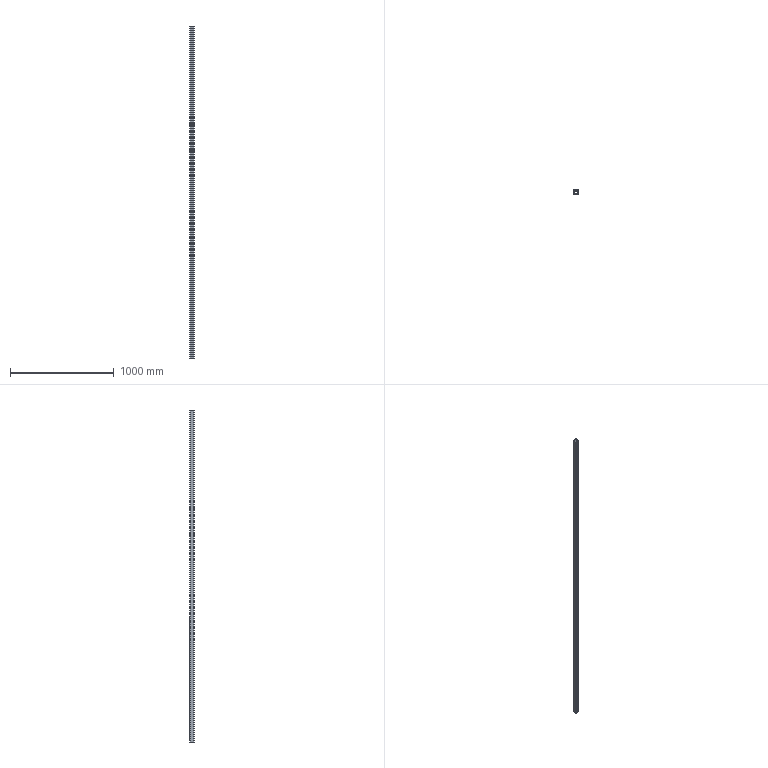Part | NX | features BREP 1 | 1 solid | 102 faces | box 40 x 42 x 3200 mm | volume 1980279 mm3 | plane 72 | cylinder 30 | commonest cylinder face diameters 2 x14 5 x10 4 x4 9 x2